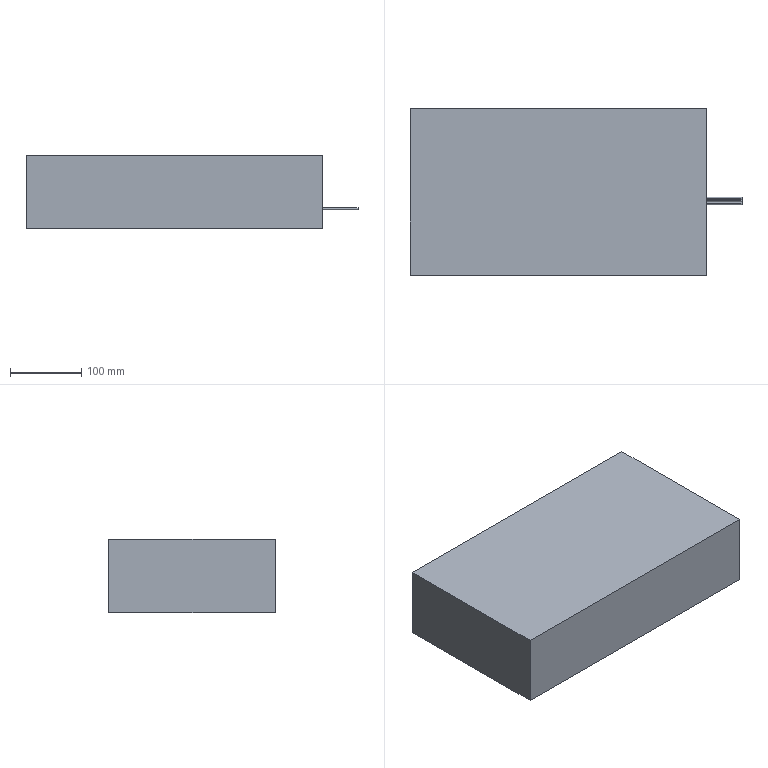Part | SolidWorks | features BaseBody 1 | 1 solid | 15 faces | box 465 x 233 x 103 mm | volume 9960645 mm3 | plane 9 | cylinder 6 | commonest cylinder face diameters 3 x6
STEP:
#1=CARTESIAN_POINT('',(162.05,-53.5,27.5));
#2=VERTEX_POINT('',#1);
#3=CARTESIAN_POINT('',(162.05,-53.5,24.5));
#4=VERTEX_POINT('',#3);
#5=CARTESIAN_POINT('',(162.05,-53.5,26.));
#6=DIRECTION('',(-1.,0.,0.));
#7=DIRECTION('',(0.,0.,1.));
#8=AXIS2_PLACEMENT_3D('',#5,#6,#7);
#9=CIRCLE('',#8,1.5);
#10=EDGE_CURVE('',#2,#4,#9,.T.);
#11=ORIENTED_EDGE('',*,*,#10,.T.);
#12=CARTESIAN_POINT('',(112.05,-53.5,24.5));
#13=VERTEX_POINT('',#12);
#14=CARTESIAN_POINT('',(162.05,-53.5,24.5));
#15=DIRECTION('',(-1.,0.,0.));
#16=VECTOR('',#15,1000.);
#17=LINE('',#14,#16);
#18=EDGE_CURVE('',#4,#13,#17,.T.);
#19=ORIENTED_EDGE('',*,*,#18,.T.);
#20=CARTESIAN_POINT('',(112.05,-53.5,27.5));
#21=VERTEX_POINT('',#20);
#22=CARTESIAN_POINT('',(112.05,-53.5,26.));
#23=DIRECTION('',(-1.,0.,0.));
#24=DIRECTION('',(0.,0.,1.));
#25=AXIS2_PLACEMENT_3D('',#22,#23,#24);
#26=CIRCLE('',#25,1.5);
#27=EDGE_CURVE('',#21,#13,#26,.T.);
#28=ORIENTED_EDGE('',*,*,#27,.F.);
#29=CARTESIAN_POINT('',(162.05,-53.5,27.5));
#30=DIRECTION('',(-1.,0.,0.));
#31=VECTOR('',#30,1000.);
#32=LINE('',#29,#31);
#33=EDGE_CURVE('',#2,#21,#32,.T.);
#34=ORIENTED_EDGE('',*,*,#33,.F.);
#35=EDGE_LOOP('',(#11,#19,#28,#34));
#36=FACE_OUTER_BOUND('',#35,.T.);
#37=CARTESIAN_POINT('',(162.05,-53.5,26.));
#38=DIRECTION('',(-1.,0.,0.));
#39=DIRECTION('',(0.,0.,1.));
#40=AXIS2_PLACEMENT_3D('',#37,#38,#39);
#41=CYLINDRICAL_SURFACE('',#40,1.5);
#42=ADVANCED_FACE('',(#36),#41,.T.);
#43=CARTESIAN_POINT('',(162.05,-60.5,27.5));
#44=VERTEX_POINT('',#43);
#45=CARTESIAN_POINT('',(162.05,-60.5,24.5));
#46=VERTEX_POINT('',#45);
#47=CARTESIAN_POINT('',(162.05,-60.5,26.));
#48=DIRECTION('',(-1.,0.,0.));
#49=DIRECTION('',(0.,0.,1.));
#50=AXIS2_PLACEMENT_3D('',#47,#48,#49);
#51=CIRCLE('',#50,1.5);
#52=EDGE_CURVE('',#44,#46,#51,.T.);
#53=ORIENTED_EDGE('',*,*,#52,.T.);
#54=CARTESIAN_POINT('',(112.05,-60.5,24.5));
#55=VERTEX_POINT('',#54);
#56=CARTESIAN_POINT('',(162.05,-60.5,24.5));
#57=DIRECTION('',(-1.,0.,0.));
#58=VECTOR('',#57,1000.);
#59=LINE('',#56,#58);
#60=EDGE_CURVE('',#46,#55,#59,.T.);
#61=ORIENTED_EDGE('',*,*,#60,.T.);
#62=CARTESIAN_POINT('',(112.05,-60.5,27.5));
#63=VERTEX_POINT('',#62);
#64=CARTESIAN_POINT('',(112.05,-60.5,26.));
#65=DIRECTION('',(-1.,0.,0.));
#66=DIRECTION('',(0.,0.,1.));
#67=AXIS2_PLACEMENT_3D('',#64,#65,#66);
#68=CIRCLE('',#67,1.5);
#69=EDGE_CURVE('',#63,#55,#68,.T.);
#70=ORIENTED_EDGE('',*,*,#69,.F.);
#71=CARTESIAN_POINT('',(162.05,-60.5,27.5));
#72=DIRECTION('',(-1.,0.,0.));
#73=VECTOR('',#72,1000.);
#74=LINE('',#71,#73);
#75=EDGE_CURVE('',#44,#63,#74,.T.);
#76=ORIENTED_EDGE('',*,*,#75,.F.);
#77=EDGE_LOOP('',(#53,#61,#70,#76));
#78=FACE_OUTER_BOUND('',#77,.T.);
#79=CARTESIAN_POINT('',(162.05,-60.5,26.));
#80=DIRECTION('',(-1.,0.,0.));
#81=DIRECTION('',(0.,0.,1.));
#82=AXIS2_PLACEMENT_3D('',#79,#80,#81);
#83=CYLINDRICAL_SURFACE('',#82,1.5);
#84=ADVANCED_FACE('',(#78),#83,.T.);
#85=CARTESIAN_POINT('',(162.05,-57.,27.5));
#86=VERTEX_POINT('',#85);
#87=CARTESIAN_POINT('',(162.05,-57.,24.5));
#88=VERTEX_POINT('',#87);
#89=CARTESIAN_POINT('',(162.05,-57.,26.));
#90=DIRECTION('',(-1.,0.,0.));
#91=DIRECTION('',(0.,0.,1.));
#92=AXIS2_PLACEMENT_3D('',#89,#90,#91);
#93=CIRCLE('',#92,1.5);
#94=EDGE_CURVE('',#86,#88,#93,.T.);
#95=ORIENTED_EDGE('',*,*,#94,.T.);
#96=CARTESIAN_POINT('',(112.05,-57.,24.5));
#97=VERTEX_POINT('',#96);
#98=CARTESIAN_POINT('',(162.05,-57.,24.5));
#99=DIRECTION('',(-1.,0.,0.));
#100=VECTOR('',#99,1000.);
#101=LINE('',#98,#100);
#102=EDGE_CURVE('',#88,#97,#101,.T.);
#103=ORIENTED_EDGE('',*,*,#102,.T.);
#104=CARTESIAN_POINT('',(112.05,-57.,27.5));
#105=VERTEX_POINT('',#104);
#106=CARTESIAN_POINT('',(112.05,-57.,26.));
#107=DIRECTION('',(-1.,0.,0.));
#108=DIRECTION('',(0.,0.,1.));
#109=AXIS2_PLACEMENT_3D('',#106,#107,#108);
#110=CIRCLE('',#109,1.5);
#111=EDGE_CURVE('',#105,#97,#110,.T.);
#112=ORIENTED_EDGE('',*,*,#111,.F.);
#113=CARTESIAN_POINT('',(162.05,-57.,27.5));
#114=DIRECTION('',(-1.,0.,0.));
#115=VECTOR('',#114,1000.);
#116=LINE('',#113,#115);
#117=EDGE_CURVE('',#86,#105,#116,.T.);
#118=ORIENTED_EDGE('',*,*,#117,.F.);
#119=EDGE_LOOP('',(#95,#103,#112,#118));
#120=FACE_OUTER_BOUND('',#119,.T.);
#121=CARTESIAN_POINT('',(162.05,-57.,26.));
#122=DIRECTION('',(-1.,0.,0.));
#123=DIRECTION('',(0.,0.,1.));
#124=AXIS2_PLACEMENT_3D('',#121,#122,#123);
#125=CYLINDRICAL_SURFACE('',#124,1.5);
#126=ADVANCED_FACE('',(#120),#125,.T.);
#127=ORIENTED_EDGE('',*,*,#94,.F.);
#128=CARTESIAN_POINT('',(162.05,-57.,26.));
#129=DIRECTION('',(-1.,0.,0.));
#130=DIRECTION('',(0.,0.,1.));
#131=AXIS2_PLACEMENT_3D('',#128,#129,#130);
#132=CIRCLE('',#131,1.5);
#133=EDGE_CURVE('',#88,#86,#132,.T.);
#134=ORIENTED_EDGE('',*,*,#133,.F.);
#135=EDGE_LOOP('',(#127,#134));
#136=FACE_OUTER_BOUND('',#135,.T.);
#137=CARTESIAN_POINT('',(162.05,-57.,26.));
#138=DIRECTION('',(1.,0.,0.));
#139=DIRECTION('',(0.,1.,0.));
#140=AXIS2_PLACEMENT_3D('',#137,#138,#139);
#141=PLANE('',#140);
#142=ADVANCED_FACE('',(#136),#141,.T.);
#143=ORIENTED_EDGE('',*,*,#52,.F.);
#144=CARTESIAN_POINT('',(162.05,-60.5,26.));
#145=DIRECTION('',(-1.,0.,0.));
#146=DIRECTION('',(0.,0.,1.));
#147=AXIS2_PLACEMENT_3D('',#144,#145,#146);
#148=CIRCLE('',#147,1.5);
#149=EDGE_CURVE('',#46,#44,#148,.T.);
#150=ORIENTED_EDGE('',*,*,#149,.F.);
#151=EDGE_LOOP('',(#143,#150));
#152=FACE_OUTER_BOUND('',#151,.T.);
#153=CARTESIAN_POINT('',(162.05,-60.5,26.));
#154=DIRECTION('',(1.,0.,0.));
#155=DIRECTION('',(0.,1.,0.));
#156=AXIS2_PLACEMENT_3D('',#153,#154,#155);
#157=PLANE('',#156);
#158=ADVANCED_FACE('',(#152),#157,.T.);
#159=ORIENTED_EDGE('',*,*,#10,.F.);
#160=CARTESIAN_POINT('',(162.05,-53.5,26.));
#161=DIRECTION('',(-1.,0.,0.));
#162=DIRECTION('',(0.,0.,1.));
#163=AXIS2_PLACEMENT_3D('',#160,#161,#162);
#164=CIRCLE('',#163,1.5);
#165=EDGE_CURVE('',#4,#2,#164,.T.);
#166=ORIENTED_EDGE('',*,*,#165,.F.);
#167=EDGE_LOOP('',(#159,#166));
#168=FACE_OUTER_BOUND('',#167,.T.);
#169=CARTESIAN_POINT('',(162.05,-53.5,26.));
#170=DIRECTION('',(1.,0.,0.));
#171=DIRECTION('',(0.,1.,0.));
#172=AXIS2_PLACEMENT_3D('',#169,#170,#171);
#173=PLANE('',#172);
#174=ADVANCED_FACE('',(#168),#173,.T.);
#175=CARTESIAN_POINT('',(-302.95,72.,101.));
#176=VERTEX_POINT('',#175);
#177=CARTESIAN_POINT('',(-302.95,-161.,101.));
#178=VERTEX_POINT('',#177);
#179=CARTESIAN_POINT('',(-302.95,0.,101.));
#180=DIRECTION('',(0.,-1.,0.));
#181=VECTOR('',#180,1000.);
#182=LINE('',#179,#181);
#183=EDGE_CURVE('',#176,#178,#182,.T.);
#184=ORIENTED_EDGE('',*,*,#183,.T.);
#185=CARTESIAN_POINT('',(112.05,-161.,101.));
#186=VERTEX_POINT('',#185);
#187=CARTESIAN_POINT('',(0.,-161.,101.));
#188=DIRECTION('',(-1.,0.,0.));
#189=VECTOR('',#188,1000.);
#190=LINE('',#187,#189);
#191=EDGE_CURVE('',#186,#178,#190,.T.);
#192=ORIENTED_EDGE('',*,*,#191,.F.);
#193=CARTESIAN_POINT('',(112.05,72.,101.));
#194=VERTEX_POINT('',#193);
#195=CARTESIAN_POINT('',(112.05,89.5,101.));
#196=DIRECTION('',(0.,-1.,0.));
#197=VECTOR('',#196,1000.);
#198=LINE('',#195,#197);
#199=EDGE_CURVE('',#194,#186,#198,.T.);
#200=ORIENTED_EDGE('',*,*,#199,.F.);
#201=CARTESIAN_POINT('',(0.,72.,101.));
#202=DIRECTION('',(1.,0.,0.));
#203=VECTOR('',#202,1000.);
#204=LINE('',#201,#203);
#205=EDGE_CURVE('',#176,#194,#204,.T.);
#206=ORIENTED_EDGE('',*,*,#205,.F.);
#207=EDGE_LOOP('',(#184,#192,#200,#206));
#208=FACE_OUTER_BOUND('',#207,.T.);
#209=CARTESIAN_POINT('',(0.,0.,101.));
#210=DIRECTION('',(0.,0.,1.));
#211=DIRECTION('',(1.,0.,0.));
#212=AXIS2_PLACEMENT_3D('',#209,#210,#211);
#213=PLANE('',#212);
#214=ADVANCED_FACE('',(#208),#213,.T.);
#215=CARTESIAN_POINT('',(-302.95,72.,-2.));
#216=VERTEX_POINT('',#215);
#217=CARTESIAN_POINT('',(112.05,72.,-2.));
#218=VERTEX_POINT('',#217);
#219=CARTESIAN_POINT('',(-217.95,72.,-2.));
#220=DIRECTION('',(1.,0.,0.));
#221=VECTOR('',#220,1000.);
#222=LINE('',#219,#221);
#223=EDGE_CURVE('',#216,#218,#222,.T.);
#224=ORIENTED_EDGE('',*,*,#223,.F.);
#225=CARTESIAN_POINT('',(-302.95,72.,0.));
#226=DIRECTION('',(0.,0.,1.));
#227=VECTOR('',#226,1000.);
#228=LINE('',#225,#227);
#229=EDGE_CURVE('',#216,#176,#228,.T.);
#230=ORIENTED_EDGE('',*,*,#229,.T.);
#231=ORIENTED_EDGE('',*,*,#205,.T.);
#232=CARTESIAN_POINT('',(112.05,72.,80.));
#233=DIRECTION('',(0.,0.,1.));
#234=VECTOR('',#233,1000.);
#235=LINE('',#232,#234);
#236=EDGE_CURVE('',#218,#194,#235,.T.);
#237=ORIENTED_EDGE('',*,*,#236,.F.);
#238=EDGE_LOOP('',(#224,#230,#231,#237));
#239=FACE_OUTER_BOUND('',#238,.T.);
#240=CARTESIAN_POINT('',(0.,72.,0.));
#241=DIRECTION('',(0.,1.,0.));
#242=DIRECTION('',(1.,0.,0.));
#243=AXIS2_PLACEMENT_3D('',#240,#241,#242);
#244=PLANE('',#243);
#245=ADVANCED_FACE('',(#239),#244,.T.);
#246=ORIENTED_EDGE('',*,*,#111,.T.);
#247=CARTESIAN_POINT('',(112.05,-57.,26.));
#248=DIRECTION('',(-1.,0.,0.));
#249=DIRECTION('',(0.,0.,1.));
#250=AXIS2_PLACEMENT_3D('',#247,#248,#249);
#251=CIRCLE('',#250,1.5);
#252=EDGE_CURVE('',#97,#105,#251,.T.);
#253=ORIENTED_EDGE('',*,*,#252,.T.);
#254=EDGE_LOOP('',(#246,#253));
#255=FACE_BOUND('',#254,.T.);
#256=ORIENTED_EDGE('',*,*,#69,.T.);
#257=CARTESIAN_POINT('',(112.05,-60.5,26.));
#258=DIRECTION('',(-1.,0.,0.));
#259=DIRECTION('',(0.,0.,1.));
#260=AXIS2_PLACEMENT_3D('',#257,#258,#259);
#261=CIRCLE('',#260,1.5);
#262=EDGE_CURVE('',#55,#63,#261,.T.);
#263=ORIENTED_EDGE('',*,*,#262,.T.);
#264=EDGE_LOOP('',(#256,#263));
#265=FACE_BOUND('',#264,.T.);
#266=ORIENTED_EDGE('',*,*,#27,.T.);
#267=CARTESIAN_POINT('',(112.05,-53.5,26.));
#268=DIRECTION('',(-1.,0.,0.));
#269=DIRECTION('',(0.,0.,1.));
#270=AXIS2_PLACEMENT_3D('',#267,#268,#269);
#271=CIRCLE('',#270,1.5);
#272=EDGE_CURVE('',#13,#21,#271,.T.);
#273=ORIENTED_EDGE('',*,*,#272,.T.);
#274=EDGE_LOOP('',(#266,#273));
#275=FACE_BOUND('',#274,.T.);
#276=CARTESIAN_POINT('',(112.05,-161.,-2.));
#277=VERTEX_POINT('',#276);
#278=CARTESIAN_POINT('',(112.05,89.5,-2.));
#279=DIRECTION('',(0.,-1.,0.));
#280=VECTOR('',#279,1000.);
#281=LINE('',#278,#280);
#282=EDGE_CURVE('',#218,#277,#281,.T.);
#283=ORIENTED_EDGE('',*,*,#282,.F.);
#284=ORIENTED_EDGE('',*,*,#236,.T.);
#285=ORIENTED_EDGE('',*,*,#199,.T.);
#286=CARTESIAN_POINT('',(112.05,-161.,0.));
#287=DIRECTION('',(0.,0.,1.));
#288=VECTOR('',#287,1000.);
#289=LINE('',#286,#288);
#290=EDGE_CURVE('',#277,#186,#289,.T.);
#291=ORIENTED_EDGE('',*,*,#290,.F.);
#292=EDGE_LOOP('',(#283,#284,#285,#291));
#293=FACE_OUTER_BOUND('',#292,.T.);
#294=CARTESIAN_POINT('',(112.05,89.5,80.));
#295=DIRECTION('',(1.,0.,0.));
#296=DIRECTION('',(0.,1.,0.));
#297=AXIS2_PLACEMENT_3D('',#294,#295,#296);
#298=PLANE('',#297);
#299=ADVANCED_FACE('',(#255,#265,#275,#293),#298,.T.);
#300=ORIENTED_EDGE('',*,*,#290,.T.);
#301=ORIENTED_EDGE('',*,*,#191,.T.);
#302=CARTESIAN_POINT('',(-302.95,-161.,-2.));
#303=VERTEX_POINT('',#302);
#304=CARTESIAN_POINT('',(-302.95,-161.,0.));
#305=DIRECTION('',(0.,0.,-1.));
#306=VECTOR('',#305,1000.);
#307=LINE('',#304,#306);
#308=EDGE_CURVE('',#178,#303,#307,.T.);
#309=ORIENTED_EDGE('',*,*,#308,.T.);
#310=CARTESIAN_POINT('',(-217.95,-161.,-2.));
#311=DIRECTION('',(-1.,0.,0.));
#312=VECTOR('',#311,1000.);
#313=LINE('',#310,#312);
#314=EDGE_CURVE('',#277,#303,#313,.T.);
#315=ORIENTED_EDGE('',*,*,#314,.F.);
#316=EDGE_LOOP('',(#300,#301,#309,#315));
#317=FACE_OUTER_BOUND('',#316,.T.);
#318=CARTESIAN_POINT('',(0.,-161.,0.));
#319=DIRECTION('',(0.,-1.,0.));
#320=DIRECTION('',(0.,0.,-1.));
#321=AXIS2_PLACEMENT_3D('',#318,#319,#320);
#322=PLANE('',#321);
#323=ADVANCED_FACE('',(#317),#322,.T.);
#324=ORIENTED_EDGE('',*,*,#229,.F.);
#325=CARTESIAN_POINT('',(-302.95,89.5,-2.));
#326=DIRECTION('',(0.,1.,0.));
#327=VECTOR('',#326,1000.);
#328=LINE('',#325,#327);
#329=EDGE_CURVE('',#303,#216,#328,.T.);
#330=ORIENTED_EDGE('',*,*,#329,.F.);
#331=ORIENTED_EDGE('',*,*,#308,.F.);
#332=ORIENTED_EDGE('',*,*,#183,.F.);
#333=EDGE_LOOP('',(#324,#330,#331,#332));
#334=FACE_OUTER_BOUND('',#333,.T.);
#335=CARTESIAN_POINT('',(-302.95,0.,0.));
#336=DIRECTION('',(1.,0.,0.));
#337=DIRECTION('',(0.,1.,0.));
#338=AXIS2_PLACEMENT_3D('',#335,#336,#337);
#339=PLANE('',#338);
#340=ADVANCED_FACE('',(#334),#339,.F.);
#341=ORIENTED_EDGE('',*,*,#314,.T.);
#342=ORIENTED_EDGE('',*,*,#329,.T.);
#343=ORIENTED_EDGE('',*,*,#223,.T.);
#344=ORIENTED_EDGE('',*,*,#282,.T.);
#345=EDGE_LOOP('',(#341,#342,#343,#344));
#346=FACE_OUTER_BOUND('',#345,.T.);
#347=CARTESIAN_POINT('',(-217.95,89.5,-2.));
#348=DIRECTION('',(0.,0.,-1.));
#349=DIRECTION('',(0.,-1.,0.));
#350=AXIS2_PLACEMENT_3D('',#347,#348,#349);
#351=PLANE('',#350);
#352=ADVANCED_FACE('',(#346),#351,.T.);
#353=ORIENTED_EDGE('',*,*,#102,.F.);
#354=ORIENTED_EDGE('',*,*,#133,.T.);
#355=ORIENTED_EDGE('',*,*,#117,.T.);
#356=ORIENTED_EDGE('',*,*,#252,.F.);
#357=EDGE_LOOP('',(#353,#354,#355,#356));
#358=FACE_OUTER_BOUND('',#357,.T.);
#359=CARTESIAN_POINT('',(162.05,-57.,26.));
#360=DIRECTION('',(-1.,0.,0.));
#361=DIRECTION('',(0.,0.,1.));
#362=AXIS2_PLACEMENT_3D('',#359,#360,#361);
#363=CYLINDRICAL_SURFACE('',#362,1.5);
#364=ADVANCED_FACE('',(#358),#363,.T.);
#365=ORIENTED_EDGE('',*,*,#60,.F.);
#366=ORIENTED_EDGE('',*,*,#149,.T.);
#367=ORIENTED_EDGE('',*,*,#75,.T.);
#368=ORIENTED_EDGE('',*,*,#262,.F.);
#369=EDGE_LOOP('',(#365,#366,#367,#368));
#370=FACE_OUTER_BOUND('',#369,.T.);
#371=CARTESIAN_POINT('',(162.05,-60.5,26.));
#372=DIRECTION('',(-1.,0.,0.));
#373=DIRECTION('',(0.,0.,1.));
#374=AXIS2_PLACEMENT_3D('',#371,#372,#373);
#375=CYLINDRICAL_SURFACE('',#374,1.5);
#376=ADVANCED_FACE('',(#370),#375,.T.);
#377=ORIENTED_EDGE('',*,*,#18,.F.);
#378=ORIENTED_EDGE('',*,*,#165,.T.);
#379=ORIENTED_EDGE('',*,*,#33,.T.);
#380=ORIENTED_EDGE('',*,*,#272,.F.);
#381=EDGE_LOOP('',(#377,#378,#379,#380));
#382=FACE_OUTER_BOUND('',#381,.T.);
#383=CARTESIAN_POINT('',(162.05,-53.5,26.));
#384=DIRECTION('',(-1.,0.,0.));
#385=DIRECTION('',(0.,0.,1.));
#386=AXIS2_PLACEMENT_3D('',#383,#384,#385);
#387=CYLINDRICAL_SURFACE('',#386,1.5);
#388=ADVANCED_FACE('',(#382),#387,.T.);
#389=CLOSED_SHELL('',(#42,#84,#126,#142,#158,#174,#214,#245,#299,#323,#340,#352,#364,#376,#388));
#390=MANIFOLD_SOLID_BREP('',#389);
#391=CARTESIAN_POINT('',(0.,0.,0.));
#392=DIRECTION('',(0.,0.,1.));
#393=DIRECTION('',(1.,0.,0.));
#394=AXIS2_PLACEMENT_3D('',#391,#392,#393);
#395=(LENGTH_UNIT()NAMED_UNIT(*)SI_UNIT(.MILLI.,.METRE.));
#396=UNCERTAINTY_MEASURE_WITH_UNIT(LENGTH_MEASURE(0.00001),#395,'','');
#397=(NAMED_UNIT(*)PLANE_ANGLE_UNIT()SI_UNIT($,.RADIAN.));
#398=(NAMED_UNIT(*)SI_UNIT($,.STERADIAN.)SOLID_ANGLE_UNIT());
#399=(GEOMETRIC_REPRESENTATION_CONTEXT(3)GLOBAL_UNCERTAINTY_ASSIGNED_CONTEXT((#396))GLOBAL_UNIT_ASSIGNED_CONTEXT((#395,#397,#398))REPRESENTATION_CONTEXT('',''));
#400=ADVANCED_BREP_SHAPE_REPRESENTATION('',(#390,#394),#399);